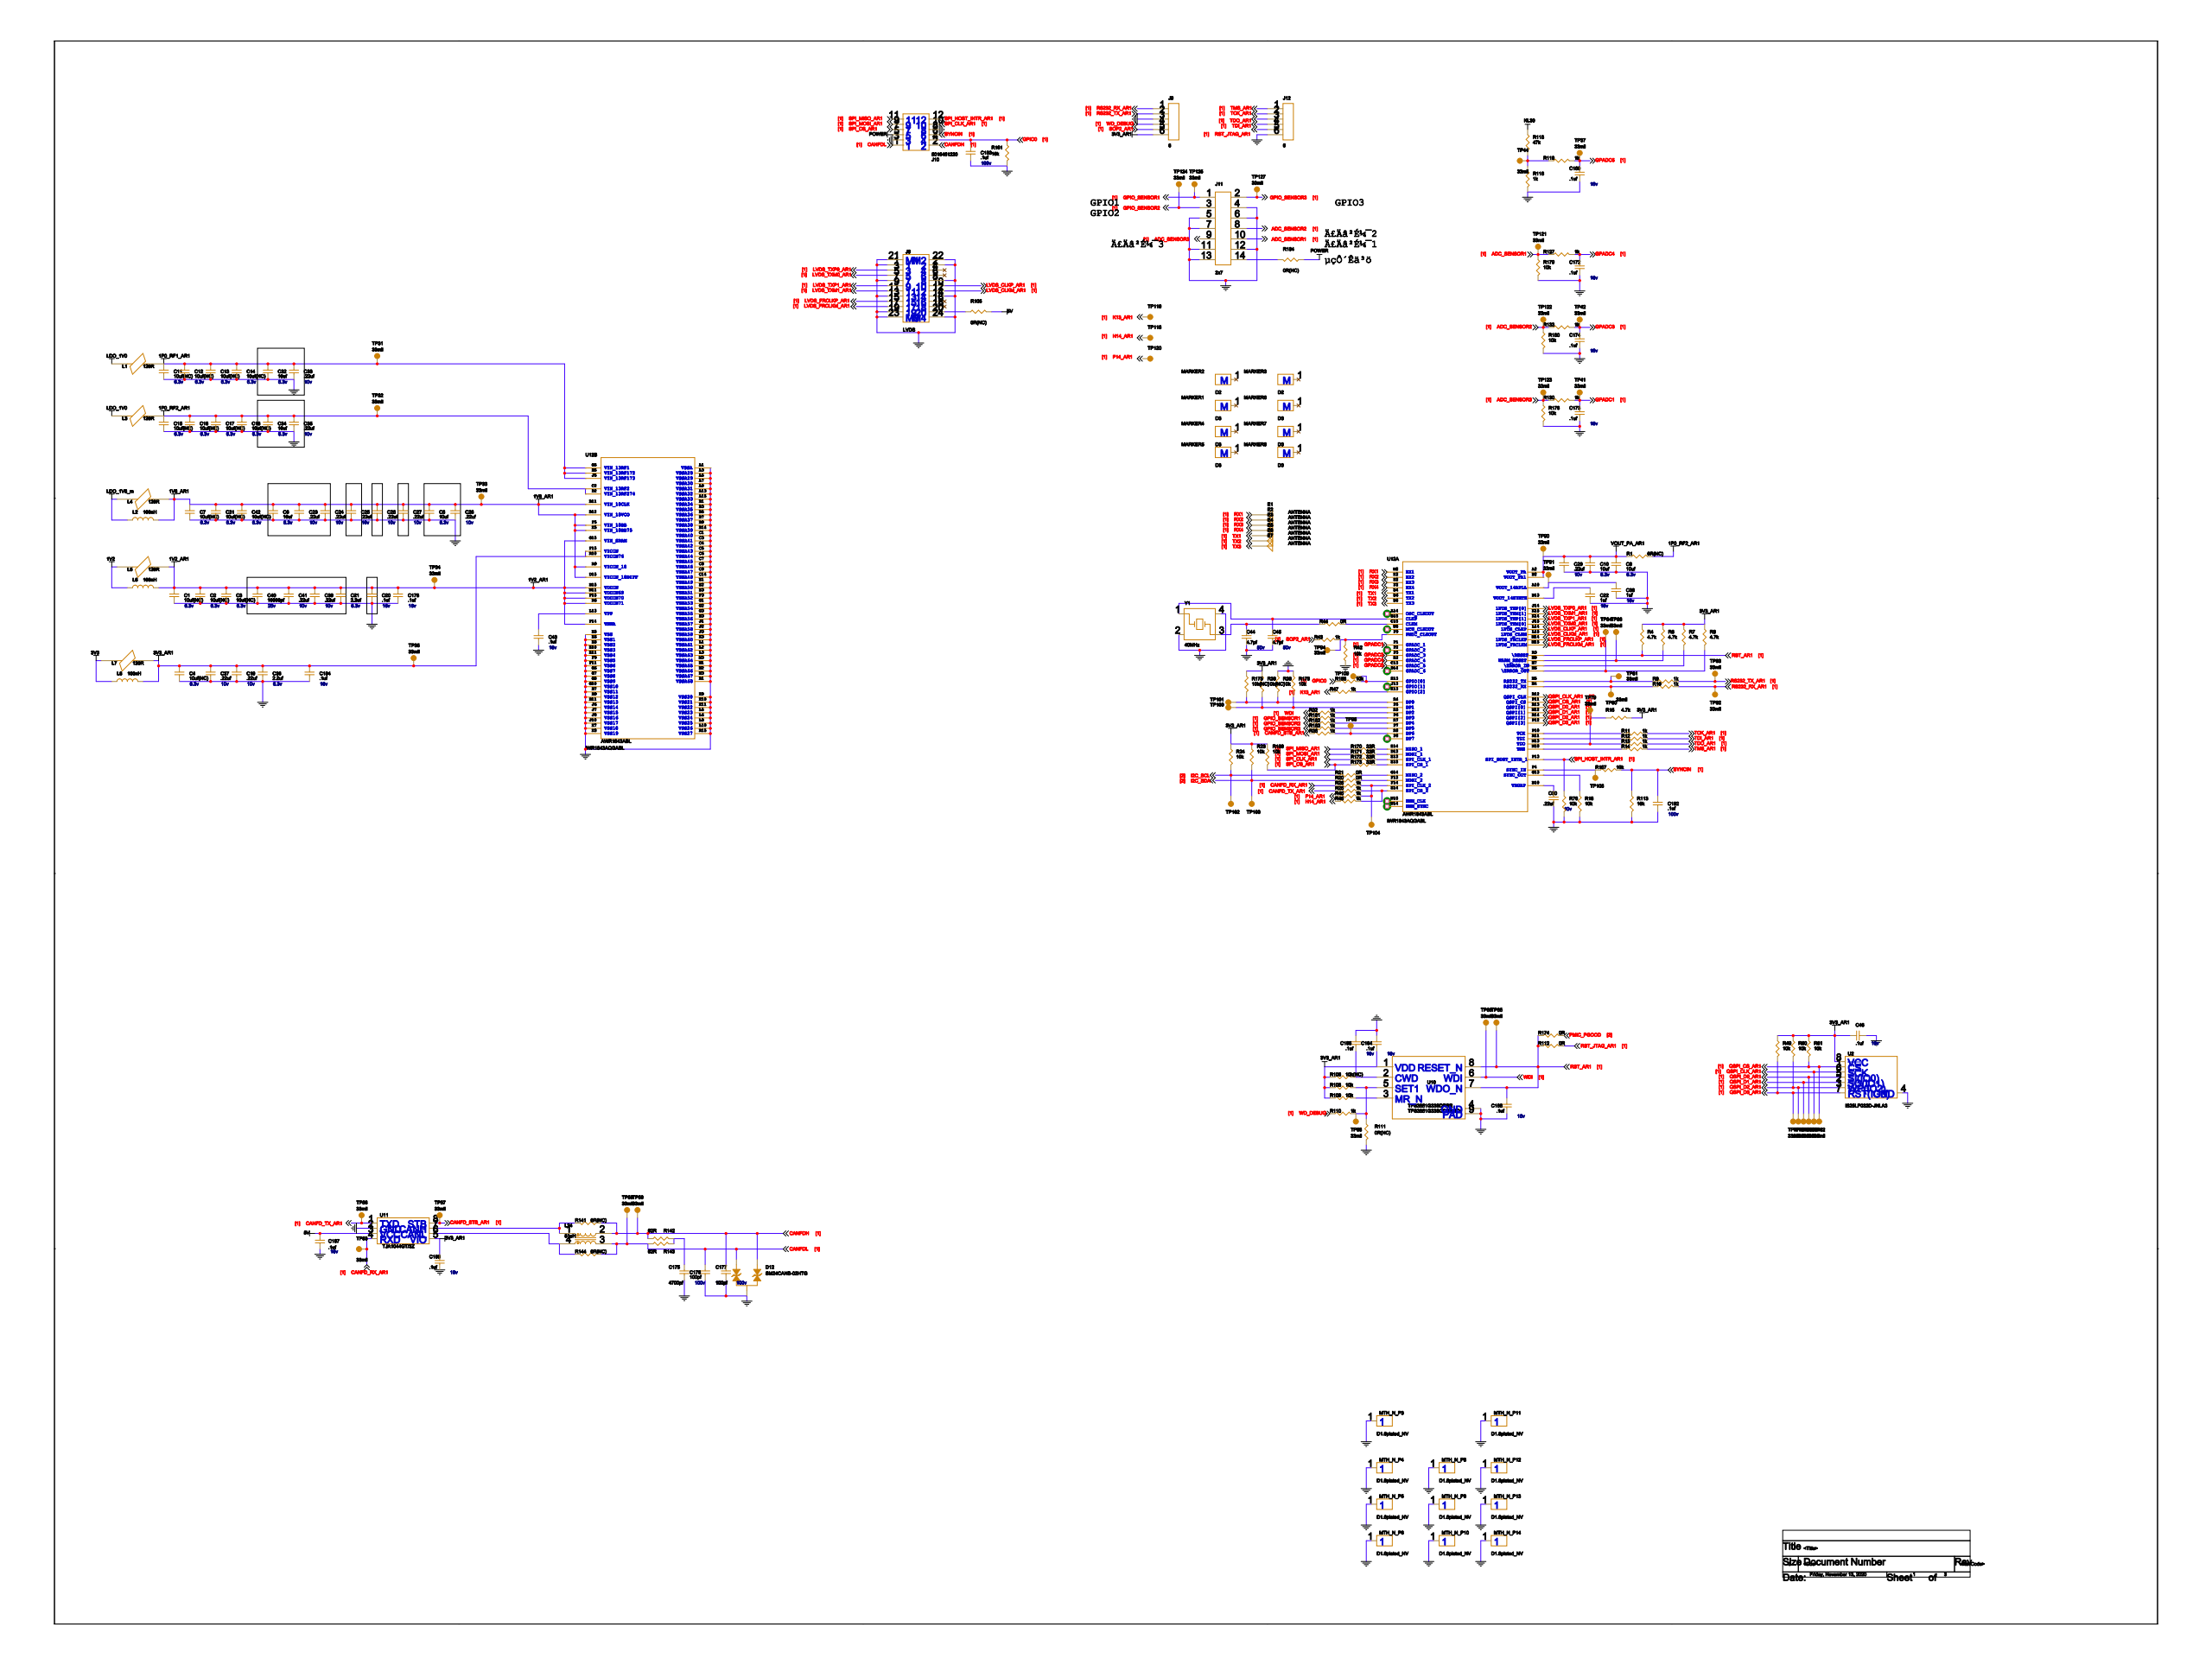Circuit board | Cadence Allegro | 338 parts | 150 nets | one sheet of the schematic
Parts on this sheet (reference | value | footprint):
C1 | 10uf(NC) | C0805
C2 | 10uf(NC) | C0805
C3 | 10uf(NC) | C0805
C4 | 10uf(NC) | C0805
C6 | 10uf | C0805
C7 | 10uf(NC) | C0805
C8 | 10uf | C0805
C9 | 10uf | C0805
C10 | 10uf | C0805
C11 | 10uf(NC) | C0805
C12 | 10uf(NC) | C0805
C13 | 10uf(NC) | C0805
C14 | 10uf(NC) | C0805
C15 | 10uf(NC) | C0805
C16 | 10uf(NC) | C0805
C17 | 10uf(NC) | C0805
C18 | 10uf(NC) | C0805
C19 | .22uf | C0402
C20 | .1uf | C0402
C21 | 2.2uf | C0603
C22 | 1uf | C0603
C23 | .22uf | C0402
C24 | .22uf | C0402
C25 | .22uf | C0402
C26 | .22uf | C0402
C27 | .22uf | C0402
C28 | .22uf | C0402
C29 | .22uf | C0402
C30 | .22uf | C0402
C31 | 10uf(NC) | C0805
C32 | 10uf | C0805
C33 | .22uf | C0402
C34 | 10uf | C0805
C35 | .22uf | C0402
C36 | 2.2uf | C0603
C37 | .22uf | C0402
C38 | 1uf | C0603
C39 | .22uf | C0402
C40 | 10000pf | C0402
C41 | .22uf | C0402
C42 | 10uf(NC) | C0805
C43 | .1uf | C0402
C44 | 4.7pf | C0402
C45 | 4.7pf | C0402
C46 | .1uf | C0402
C164 | .1uf | C0402
C165 | .1uf | C0402
C166 | .1uf | C0402
C167 | .1uf | C0402
C168 | .1uf | C0402
C169 | .1uf | C0402
C172 | .1uf | C0402
C173 | .1uf | C0402
C174 | .1uf | C0402
C175 | 4700pf | C0603
C176 | 100pf | C0603
C177 | 100pf | C0603
C178 | .1uf | C0402
C182 | .1uf | C0805
C183 | .1uf | C0805
C184 | .1uf | C0402
D12 | SM24CANB-02HTG | SOT23
E1 | ANTENNA | ANTENNA
E2 | ANTENNA | ANTENNA
E3 | ANTENNA | ANTENNA
E4 | ANTENNA | ANTENNA
E5 | ANTENNA | ANTENNA
E6 | ANTENNA | ANTENNA
E7 | ANTENNA | ANTENNA
J6 | LVDS | LVDS
J9 | 6 | TST6X254
J10 | 5016451220 | 5016451220
J11 | 2x7 | CON2X7X200
J12 | 6 | TST6X254
L1 | 120R | L0603
L2 | 100nH | NLCV32T-R10M-EFRD
L3 | 120R | L0603
L4 | 120R | L0603
L5 | 120R | L0603
L6 | 100nH | NLCV32T-R10M-EFRD
L7 | 120R | L0603
L8 | 100nH | NLCV32T-R10M-EFRD
L24 | 51uH | CM320X450X150-4N
MTH_N_P3 | D1.6plated_NV | MTGP200H160P
MTH_N_P4 | D1.6plated_NV | MTGP200H160P
MTH_N_P5 | D1.6plated_NV | MTGP200H160P
MTH_N_P6 | D1.6plated_NV | MTGP200H160P
MTH_N_P8 | D1.6plated_NV | MTGP200H160P
MTH_N_P9 | D1.6plated_NV | MTGP200H160P
MTH_N_P10 | D1.6plated_NV | MTGP200H160P
MTH_N_P11 | D1.6plated_NV | MTGP200H160P
MTH_N_P12 | D1.6plated_NV | MTGP200H160P
MTH_N_P13 | D1.6plated_NV | MTGP200H160P
MTH_N_P14 | D1.6plated_NV | MTGP200H160P
R1 | 0R(NC) | R0603
R4 | 4.7k | R0402
R6 | 4.7k | R0402
R7 | 4.7k | R0402
R8 | 4.7k | R0402
R9 | 1k | R0402
R10 | 1k | R0402
R11 | 1k | R0402
R12 | 1k | R0402
R13 | 1k | R0402
R14 | 1k | R0402
R15 | 4.7k | R0402
R18 | 10k | R0402
R20 | 0R | R0402
R21 | 0R | R0402
R23 | 10k | R0402
R24 | 10k | R0402
R25 | 1k | R0402
R26 | 1k | R0402
R32 | 1k | R0402
R36 | 1k | R0402
R38 | 10k | R0402
R39 | 10k(NC) | R0402
R42 | 10k | R0402
R43 | 1k | R0402
R44 | 0R | R0402
R45 | 1k | R0402
R46 | 1k | R0402
R47 | 1k | R0402
R49 | 10k | R0402
R50 | 10k | R0402
R51 | 10k | R0402
R76 | 10k | R0402
R105 | 0R(NC) | R0603
R106 | 10k(NC) | R0402
R108 | 10k | R0402
R109 | 10k | R0402
R110 | 1k | R0402
R111 | 0R(NC) | R0402
R112 | 0R | R0402
R113 | 10k | R0402
R116 | 1k | R0402
R118 | 47k | R0402
R119 | 1k | R0402
R127 | 1k | R0402
R130 | 1k | R0402
R133 | 1k | R0402
R141 | 0R(NC) | R0402
R142 | 62R | R1206
R143 | 62R | R1206
R144 | 0R(NC) | R0402
R161 | 10k | R0402
R167 | 10k | R0402
R168 | 10k | R0402
R169 | 10k | R0402
R170 | 33R | R0402
R171 | 33R | R0402
R172 | 33R | R0402
R173 | 33R | R0402
R174 | 0R | R0402
R175 | 10k(NC) | R0402
R176 | 10k | R0402
R178 | 10k | R0402
R179 | 10k | R0402
R180 | 10k | R0402
R181 | 1k | R0402
R182 | 1k | R0402
R183 | 1k | R0402
R184 | 0R(NC) | R0805
TP31 | 33mil | TPAD_33MIL
TP32 | 33mil | TPAD_33MIL
TP33 | 33mil | TPAD_33MIL
TP34 | 33mil | TPAD_33MIL
TP35 | 33mil | TPAD_33MIL
TP37 | 33mil | TPAD_33MIL
TP41 | 33mil | TPAD_33MIL
TP42 | 33mil | TPAD_33MIL
TP44 | 33mil | TPAD_33MIL
TP47 | 33mil | TPAD_33MIL
TP48 | 33mil | TPAD_33MIL
TP49 | 33mil | TPAD_33MIL
TP50 | 33mil | TPAD_33MIL
TP51 | 33mil | TPAD_33MIL
TP52 | 33mil | TPAD_33MIL
TP53 | 33mil | TPAD_33MIL
TP56 | 33mil | TPAD_33MIL
TP57 | 33mil | TPAD_33MIL
TP58 | 33mil | TPAD_33MIL
TP59 | 33mil | TPAD_33MIL
TP65 | 33mil | TPAD_33MIL
TP66 | 33mil | TPAD_33MIL
TP68 | 33mil | TPAD_33MIL
TP79 | 33mil | TPAD_33MIL
TP80 | 33mil | TPAD_33MIL
TP81 | 33mil | TPAD_33MIL
TP82 | 33mil | TPAD_33MIL
TP83 | 33mil | TPAD_33MIL
TP84 | 33mil | TPAD_33MIL
TP86 | 33mil | TPAD_33MIL
TP90 | 33mil | TPAD_33MIL
TP91 | 33mil | TPAD_33MIL
TP94 | 33mil | TPAD_33MIL
TP95 | 33mil | TPAD_33MIL
TP100 | 33mil | TPAD_33MIL
TP101 | 33mil | TPAD_33MIL
TP102 | 33mil | TPAD_33MIL
TP103 | 33mil | TPAD_33MIL
TP104 | 33mil | TPAD_33MIL
TP108 | 33mil | TPAD_33MIL
TP109 | 33mil | TPAD_33MIL
TP118 | debug | TST1
TP119 | debug | TST1
TP120 | debug | TST1
TP121 | 33mil | TPAD_33MIL
TP122 | 33mil | TPAD_33MIL
TP123 | 33mil | TPAD_33MIL
TP124 | 33mil | TPAD_33MIL
TP125 | 33mil | TPAD_33MIL
TP127 | 33mil | TPAD_33MIL
U2 | IS25LP032D-JNLA3 | SOIC127P600X175-8N
U10 | TPS3851G33SQDRBRQ1 | DRB0008A
U11 | TJA1044GT/3Z | SOIC127P600X175-8N
U12 | IWR1843AQGABL | ABL0161B
Y1 | 40MHz | OSCCC250X320X85-4N
Nets of these parts (net: part-pin ...):
KL30: R118-1
POWER: J10-5 R184-1
N664061: J11-14 R184-2
PMIC_PGOOD: R174-2
GPIO_SENSOR1: J11-1 R181-1 TP125-1
ADC_SENSOR1: J11-10 R127-1 R179-1 TP121-1
GND: C1-2 C2-2 C3-2 C4-2 C6-2 C7-2 C8-2 C9-2 C10-2 C11-2 C12-2 C13-2 C14-2 C15-2 C16-2 C17-2 C18-2 C19-2 C20-2 C21-2 C22-2 C23-2 C24-2 C25-2 C26-2 C27-2 C28-2 C29-2 C30-2 C31-2 C32-2 C33-2 C34-2 C35-2 C36-2 C37-2 C38-2 C39-2 C40-2 C41-2 C42-2 C43-2 C44-2 C45-2 C46-2 C164-1 C165-1 C166-2 C167-1 C168-2 C169-2 C172-2 C173-2 C174-2 C175-2 C176-2 C177-2 C178-2 C182-2 C183-2 C184-2 D12-3 J6-1 J6-2 J6-7 J6-8 J6-13 J6-14 J6-19 J6-21 J6-22 J6-23 J6-24 J9-3 J10-3 J10-8 J11-4 J11-5 J11-6 J11-7 J11-11 J11-12 J11-13 J12-6 MTH_N_P3-1 MTH_N_P4-1 MTH_N_P5-1 MTH_N_P6-1 MTH_N_P8-1 MTH_N_P9-1 MTH_N_P10-1 MTH_N_P11-1 MTH_N_P12-1 MTH_N_P13-1 MTH_N_P14-1 R18-2 R38-1 R42-1 R76-2 R111-2 R113-2 R116-2 R161-2 R176-1 R178-2 R179-2 R180-2 U2-4 U10-4 U10-9 U11-2 Y1-2 Y1-4 U12-A1 U12-A3 U12-A5 U12-A7 U12-A9 U12-A13 U12-A15 U12-B1 U12-B3 U12-B5 U12-B7 U12-B9 U12-B14 U12-C1 U12-C3 U12-C4 U12-C5 U12-C6 U12-C7 U12-C8 U12-C9 U12-C14 U12-E1 U12-E2 U12-E3 U12-E5 U12-E6 U12-E8 U12-E10 U12-E11 U12-F3 U12-F9 U12-F11 U12-G1 U12-G2 U12-G3 U12-G6 U12-G7 U12-G8 U12-G10 U12-H3 U12-H7 U12-H9 U12-H11 U12-J1 U12-J2 U12-J3 U12-J6 U12-J7 U12-J8 U12-J10 U12-K3 U12-K7 U12-K8 U12-K9 U12-K10 U12-K11 U12-L1 U12-L2 U12-L3 U12-L5 U12-L6 U12-L8 U12-L10 U12-M3 U12-N1 U12-N2 U12-N3 U12-R1 U12-R15
GPIO_SENSOR3: J11-2 R183-1 TP127-1
GPIO_SENSOR2: J11-3 R182-1 TP124-1
ADC_SENSOR2: J11-8 R133-1 R180-1 TP122-1
ADC_SENSOR3: J11-9 R130-1 R178-1 TP123-1
1V2_AR1: C1-1 C2-1 C3-1 C20-1 C21-1 C39-1 C40-1 C41-1 C178-1 L5-2 L6-2 TP34-1 U12-G15 U12-H15 U12-N11 U12-P14 U12-P15 U12-R6
1P0_RF1_AR1: C11-1 C12-1 C13-1 C14-1 C32-1 C33-1 L1-2 TP31-1 U12-G5 U12-H5 U12-J5
1P0_RF2_AR1: C15-1 C16-1 C17-1 C18-1 C34-1 C35-1 L3-2 R1-2 TP32-1 U12-C2 U12-D2
1V8_AR1: C6-1 C7-1 C8-1 C23-1 C24-1 C25-1 C26-1 C27-1 C28-1 C31-1 C42-1 L2-2 L4-2 TP33-1 U12-B11 U12-B12 U12-D15 U12-F5 U12-K5 U12-R9
3V3_AR1: C4-1 C19-1 C36-1 C37-1 C46-1 C164-2 C168-1 C184-1 J9-6 L7-2 L8-2 R4-1 R6-1 R7-1 R8-1 R15-2 R23-1 R24-1 R39-1 R49-1 R50-1 R51-1 R106-1 R108-1 R109-1 R169-1 R175-1 TP35-1 U2-8 U10-1 U11-5 U12-F15 U12-R10
TMS_AR1: J12-1 R14-2
TCK_AR1: J12-2 R11-2
TDO_AR1: J12-3 R13-2
TDI_AR1: J12-4 R12-2
RST_JTAG_AR1: J12-5 R112-2
RS232_RX_AR1: J9-1 R10-2 TP82-1
RS232_TX_AR1: J9-2 R9-2 TP83-1
WD_DEBUG: J9-4 R110-1
SOP2_AR1: J9-5 R43-1
SPI_MISO_AR1: J10-11 R170-1
N582573: R170-2 U12-E14
SPI_MOSI_AR1: J10-9 R171-1
N582607: R171-2 U12-D13
SPI_CLK_AR1: J10-10 R172-1
N582637: R172-2 U12-E13
SPI_CS_AR1: J10-7 R169-2 R173-1
N582669: R173-2 U12-E15
3V3: L7-1 L8-1
1V2: L5-1 L6-1
5V: C167-2 R105-2 U11-3
LDO_1V0: L1-1 L3-1
CANFDL: C176-1 D12-2 J10-1 L24-3 R143-1 R144-1 TP58-1
SPI_HOST_INTR_AR1: J10-12 R76-1 U12-P13
CANFDH: C177-1 D12-1 J10-2 L24-2 R141-1 R142-1 TP59-1
GPIO0: C183-1 J10-4 R161-1 R168-1
SYNCIN: C182-1 J10-6 R113-1 R167-2
H14_AR1: R46-1 TP118-1
K13_AR1: R47-1 TP119-1
F14_AR1: R45-1 TP120-1
LDO_1V8_M: L2-1 L4-1
RX1: E1-1 U12-M2
RX2: E2-1 U12-K2
RX3: E3-1 U12-H2
RX4: E4-1 U12-F2
TX1: E5-1 U12-B4
TX2: E6-1 U12-B6
TX3: E7-1 U12-B8
VOUT_PA_AR1: C9-1 C10-1 C29-1 R1-1 TP90-1 U12-A2 U12-B2
N138496: C165-2 R106-2 U10-2
RST_AR1: C166-1 R4-2 R112-1 R174-1 TP65-1 U10-7 U10-8 U12-R3
GPADC5: C169-1 R119-2 TP37-1 U12-C13
GPADC4: C172-1 R127-2 U12-R2
GPADC1: C173-1 R130-2 TP41-1 U12-P1
GPADC3: C174-1 R133-2 TP42-1 U12-P3
N08770: C43-1 U12-L13
N07239: C30-1 U12-B10
N158757: C175-1 R142-2 R143-2
N07911: C22-1 U12-B13
N07899: C38-1 TP91-1 U12-A10
N17024: C44-1 R44-1 Y1-3
N17037: C45-1 Y1-1 U12-B15
LVDS_CLKP_AR1: J6-10 U12-L14
LVDS_TXM1_AR1: J6-11 U12-K15
LVDS_CLKM_AR1: J6-12 U12-L15
LVDS_FRCLKP_AR1: J6-15 U12-M14
LVDS_FRCLKM_AR1: J6-17 U12-M15
N133595: J6-20 R105-1
LVDS_TXP0_AR1: J6-3 U12-J14
LVDS_TXM0_AR1: J6-5 U12-J15
LVDS_TXP1_AR1: J6-9 U12-K14
N158641: L24-1 R141-2 U11-7
N158769: L24-4 R144-2 U11-6
N637865: R181-2 U12-P6
N637869: R182-2 U12-R7
N637873: R183-2 U12-P7
N14430: R10-1 TP80-1 U12-N4
N14660: R11-1 U12-P10
N135788: R108-2 R110-2 R111-1 TP68-1 U10-5
N151263: R116-1 R118-2 R119-1 TP44-1
N14818: R12-1 U12-R11
N14816: R13-1 R15-1 TP79-1 U12-N13
N14814: R14-1 U12-N10
CANFD_TX_AR1: R25-1 TP56-1 U11-1
N15788: R25-2 R46-2 U12-H14
CANFD_RX_AR1: R26-1 TP53-1 U11-4
N15786: R26-2 R45-2 TP104-1 U12-F14
WDI: R32-1 TP66-1 U10-6
N16125: R32-2 U12-R5
CANFD_STB_AR1: R36-1 TP57-1 U11-8
N16135: R36-2 TP95-1 U12-R8
N23649: R42-2 R43-2 TP94-1 U12-P9
N26356: R47-2 U12-K13
N14408: R9-1 TP81-1 U12-N5
N16123: R39-2 R176-2 TP100-1 U12-P5
N16133: R38-2 R175-2 TP101-1 U12-R4
N15068: R167-1 TP108-1 U12-P4
N435439: R168-2 TP109-1 U12-H13
N135786: R109-2 U10-3
N15072: R18-1 U12-G13
I2C_SDA: R20-1 R23-2 TP103-1
I2C_SCL: R21-1 R24-2 TP102-1
QSPI_D3_AR1: R49-2 TP47-1 U2-7 U12-P12
QSPI_D2_AR1: R50-2 TP48-1 U2-3 U12-R14
QSPI_CS_AR1: R51-2 TP52-1 U2-1 U12-P11
N15443: R20-2 U12-F13
N15441: R21-2 U12-G14
N25661: R44-2 U12-C15
N14212: R6-2 TP86-1 U12-N9
N14216: R7-2 U12-N7
N14220: R8-2 TP84-1 U12-N6
QSPI_D1_AR1: TP49-1 U2-2 U12-N12
QSPI_D0_AR1: TP50-1 U2-5 U12-R13
QSPI_CLK_AR1: TP51-1 U2-6 U12-R12